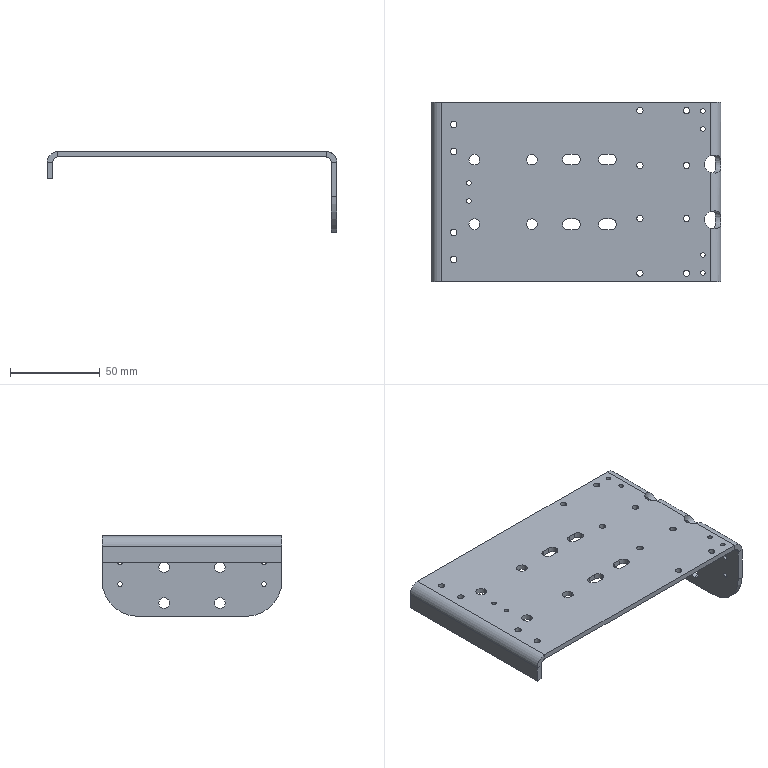Part | STEP file | Lead screw guide rail connecting plate split 2V1.201001 | 1 solid | 108 faces | box 161 x 100 x 44.931 mm | volume 60540 mm3 | cylinder 80 | plane 26 | spline 2 | commonest cylinder face diameters 6 x30 3.5 x24 2.5 x20 10 x2 12 x2 40 x2